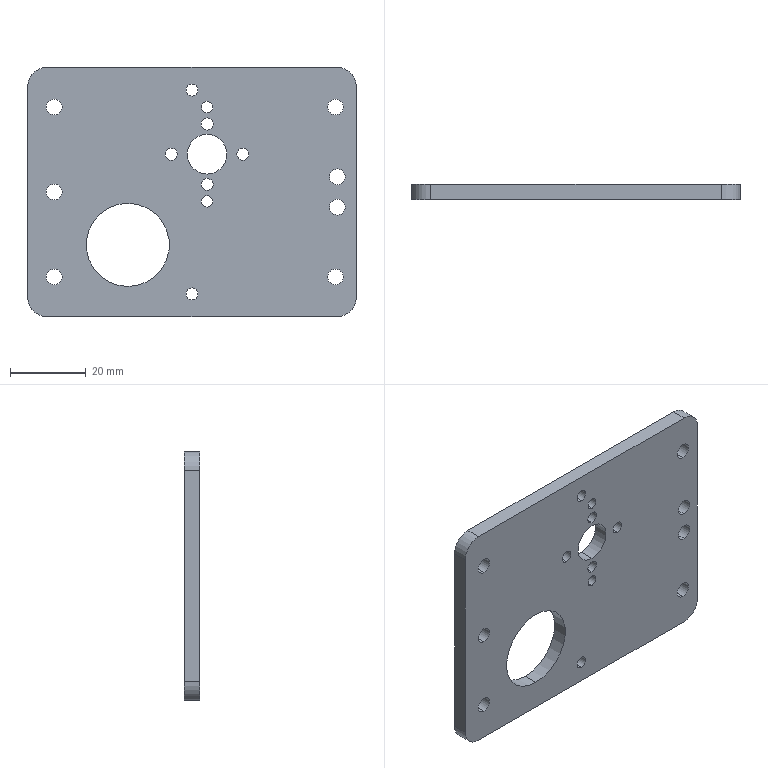Part | SolidWorks | features BaseBody 1 | 1 solid | 44 faces | box 87 x 4 x 66 mm | volume 20378 mm3 | cylinder 38 | plane 6 | commonest cylinder face diameters 4.2 x14 3.2 x12 3 x4 10 x4 10.5 x2 22 x2
STEP:
#1=CARTESIAN_POINT('',(38.5,4.,6.1));
#2=VERTEX_POINT('',#1);
#3=CARTESIAN_POINT('',(38.5,4.,1.9));
#4=VERTEX_POINT('',#3);
#5=CARTESIAN_POINT('',(38.5,4.,4.));
#6=DIRECTION('',(0.,-1.,0.));
#7=DIRECTION('',(0.,0.,-1.));
#8=AXIS2_PLACEMENT_3D('',#5,#6,#7);
#9=CIRCLE('',#8,2.1);
#10=EDGE_CURVE('',#2,#4,#9,.T.);
#11=ORIENTED_EDGE('',*,*,#10,.F.);
#12=CARTESIAN_POINT('',(38.5,0.,6.1));
#13=VERTEX_POINT('',#12);
#14=CARTESIAN_POINT('',(38.5,4.,6.1));
#15=DIRECTION('',(0.,-1.,0.));
#16=VECTOR('',#15,1000.);
#17=LINE('',#14,#16);
#18=EDGE_CURVE('',#2,#13,#17,.T.);
#19=ORIENTED_EDGE('',*,*,#18,.T.);
#20=CARTESIAN_POINT('',(38.5,0.,1.9));
#21=VERTEX_POINT('',#20);
#22=CARTESIAN_POINT('',(38.5,0.,4.));
#23=DIRECTION('',(0.,1.,0.));
#24=DIRECTION('',(0.,0.,-1.));
#25=AXIS2_PLACEMENT_3D('',#22,#23,#24);
#26=CIRCLE('',#25,2.1);
#27=EDGE_CURVE('',#21,#13,#26,.T.);
#28=ORIENTED_EDGE('',*,*,#27,.F.);
#29=CARTESIAN_POINT('',(38.5,4.,1.9));
#30=DIRECTION('',(0.,-1.,0.));
#31=VECTOR('',#30,1000.);
#32=LINE('',#29,#31);
#33=EDGE_CURVE('',#4,#21,#32,.T.);
#34=ORIENTED_EDGE('',*,*,#33,.F.);
#35=EDGE_LOOP('',(#11,#19,#28,#34));
#36=FACE_OUTER_BOUND('',#35,.T.);
#37=CARTESIAN_POINT('',(38.5,4.,4.));
#38=DIRECTION('',(0.,-1.,0.));
#39=DIRECTION('',(0.,0.,-1.));
#40=AXIS2_PLACEMENT_3D('',#37,#38,#39);
#41=CYLINDRICAL_SURFACE('',#40,2.1);
#42=ADVANCED_FACE('',(#36),#41,.F.);
#43=CARTESIAN_POINT('',(38.5,4.,-1.9));
#44=VERTEX_POINT('',#43);
#45=CARTESIAN_POINT('',(38.5,4.,-6.1));
#46=VERTEX_POINT('',#45);
#47=CARTESIAN_POINT('',(38.5,4.,-4.));
#48=DIRECTION('',(0.,-1.,0.));
#49=DIRECTION('',(0.,0.,-1.));
#50=AXIS2_PLACEMENT_3D('',#47,#48,#49);
#51=CIRCLE('',#50,2.1);
#52=EDGE_CURVE('',#44,#46,#51,.T.);
#53=ORIENTED_EDGE('',*,*,#52,.F.);
#54=CARTESIAN_POINT('',(38.5,0.,-1.9));
#55=VERTEX_POINT('',#54);
#56=CARTESIAN_POINT('',(38.5,4.,-1.9));
#57=DIRECTION('',(0.,-1.,0.));
#58=VECTOR('',#57,1000.);
#59=LINE('',#56,#58);
#60=EDGE_CURVE('',#44,#55,#59,.T.);
#61=ORIENTED_EDGE('',*,*,#60,.T.);
#62=CARTESIAN_POINT('',(38.5,0.,-6.1));
#63=VERTEX_POINT('',#62);
#64=CARTESIAN_POINT('',(38.5,0.,-4.));
#65=DIRECTION('',(0.,1.,0.));
#66=DIRECTION('',(0.,0.,-1.));
#67=AXIS2_PLACEMENT_3D('',#64,#65,#66);
#68=CIRCLE('',#67,2.1);
#69=EDGE_CURVE('',#63,#55,#68,.T.);
#70=ORIENTED_EDGE('',*,*,#69,.F.);
#71=CARTESIAN_POINT('',(38.5,4.,-6.1));
#72=DIRECTION('',(0.,-1.,0.));
#73=VECTOR('',#72,1000.);
#74=LINE('',#71,#73);
#75=EDGE_CURVE('',#46,#63,#74,.T.);
#76=ORIENTED_EDGE('',*,*,#75,.F.);
#77=EDGE_LOOP('',(#53,#61,#70,#76));
#78=FACE_OUTER_BOUND('',#77,.T.);
#79=CARTESIAN_POINT('',(38.5,4.,-4.));
#80=DIRECTION('',(0.,-1.,0.));
#81=DIRECTION('',(0.,0.,-1.));
#82=AXIS2_PLACEMENT_3D('',#79,#80,#81);
#83=CYLINDRICAL_SURFACE('',#82,2.1);
#84=ADVANCED_FACE('',(#78),#83,.F.);
#85=CARTESIAN_POINT('',(0.,4.,28.6));
#86=VERTEX_POINT('',#85);
#87=CARTESIAN_POINT('',(0.,4.,25.4));
#88=VERTEX_POINT('',#87);
#89=CARTESIAN_POINT('',(0.,4.,27.));
#90=DIRECTION('',(0.,-1.,0.));
#91=DIRECTION('',(0.,0.,-1.));
#92=AXIS2_PLACEMENT_3D('',#89,#90,#91);
#93=CIRCLE('',#92,1.6);
#94=EDGE_CURVE('',#86,#88,#93,.T.);
#95=ORIENTED_EDGE('',*,*,#94,.F.);
#96=CARTESIAN_POINT('',(0.,0.,28.6));
#97=VERTEX_POINT('',#96);
#98=CARTESIAN_POINT('',(0.,4.,28.6));
#99=DIRECTION('',(0.,-1.,0.));
#100=VECTOR('',#99,1000.);
#101=LINE('',#98,#100);
#102=EDGE_CURVE('',#86,#97,#101,.T.);
#103=ORIENTED_EDGE('',*,*,#102,.T.);
#104=CARTESIAN_POINT('',(0.,0.,25.4));
#105=VERTEX_POINT('',#104);
#106=CARTESIAN_POINT('',(0.,0.,27.));
#107=DIRECTION('',(0.,1.,0.));
#108=DIRECTION('',(0.,0.,-1.));
#109=AXIS2_PLACEMENT_3D('',#106,#107,#108);
#110=CIRCLE('',#109,1.6);
#111=EDGE_CURVE('',#105,#97,#110,.T.);
#112=ORIENTED_EDGE('',*,*,#111,.F.);
#113=CARTESIAN_POINT('',(0.,4.,25.4));
#114=DIRECTION('',(0.,-1.,0.));
#115=VECTOR('',#114,1000.);
#116=LINE('',#113,#115);
#117=EDGE_CURVE('',#88,#105,#116,.T.);
#118=ORIENTED_EDGE('',*,*,#117,.F.);
#119=EDGE_LOOP('',(#95,#103,#112,#118));
#120=FACE_OUTER_BOUND('',#119,.T.);
#121=CARTESIAN_POINT('',(0.,4.,27.));
#122=DIRECTION('',(0.,-1.,0.));
#123=DIRECTION('',(0.,0.,-1.));
#124=AXIS2_PLACEMENT_3D('',#121,#122,#123);
#125=CYLINDRICAL_SURFACE('',#124,1.6);
#126=ADVANCED_FACE('',(#120),#125,.F.);
#127=CARTESIAN_POINT('',(38.,4.,-20.4));
#128=VERTEX_POINT('',#127);
#129=CARTESIAN_POINT('',(38.,4.,-24.6));
#130=VERTEX_POINT('',#129);
#131=CARTESIAN_POINT('',(38.,4.,-22.5));
#132=DIRECTION('',(0.,-1.,0.));
#133=DIRECTION('',(0.,0.,-1.));
#134=AXIS2_PLACEMENT_3D('',#131,#132,#133);
#135=CIRCLE('',#134,2.1);
#136=EDGE_CURVE('',#128,#130,#135,.T.);
#137=ORIENTED_EDGE('',*,*,#136,.F.);
#138=CARTESIAN_POINT('',(38.,0.,-20.4));
#139=VERTEX_POINT('',#138);
#140=CARTESIAN_POINT('',(38.,4.,-20.4));
#141=DIRECTION('',(0.,-1.,0.));
#142=VECTOR('',#141,1000.);
#143=LINE('',#140,#142);
#144=EDGE_CURVE('',#128,#139,#143,.T.);
#145=ORIENTED_EDGE('',*,*,#144,.T.);
#146=CARTESIAN_POINT('',(38.,0.,-24.6));
#147=VERTEX_POINT('',#146);
#148=CARTESIAN_POINT('',(38.,0.,-22.5));
#149=DIRECTION('',(0.,1.,0.));
#150=DIRECTION('',(0.,0.,-1.));
#151=AXIS2_PLACEMENT_3D('',#148,#149,#150);
#152=CIRCLE('',#151,2.1);
#153=EDGE_CURVE('',#147,#139,#152,.T.);
#154=ORIENTED_EDGE('',*,*,#153,.F.);
#155=CARTESIAN_POINT('',(38.,4.,-24.6));
#156=DIRECTION('',(0.,-1.,0.));
#157=VECTOR('',#156,1000.);
#158=LINE('',#155,#157);
#159=EDGE_CURVE('',#130,#147,#158,.T.);
#160=ORIENTED_EDGE('',*,*,#159,.F.);
#161=EDGE_LOOP('',(#137,#145,#154,#160));
#162=FACE_OUTER_BOUND('',#161,.T.);
#163=CARTESIAN_POINT('',(38.,4.,-22.5));
#164=DIRECTION('',(0.,-1.,0.));
#165=DIRECTION('',(0.,0.,-1.));
#166=AXIS2_PLACEMENT_3D('',#163,#164,#165);
#167=CYLINDRICAL_SURFACE('',#166,2.1);
#168=ADVANCED_FACE('',(#162),#167,.F.);
#169=CARTESIAN_POINT('',(38.,4.,24.6));
#170=VERTEX_POINT('',#169);
#171=CARTESIAN_POINT('',(38.,4.,20.4));
#172=VERTEX_POINT('',#171);
#173=CARTESIAN_POINT('',(38.,4.,22.5));
#174=DIRECTION('',(0.,-1.,0.));
#175=DIRECTION('',(0.,0.,-1.));
#176=AXIS2_PLACEMENT_3D('',#173,#174,#175);
#177=CIRCLE('',#176,2.1);
#178=EDGE_CURVE('',#170,#172,#177,.T.);
#179=ORIENTED_EDGE('',*,*,#178,.F.);
#180=CARTESIAN_POINT('',(38.,0.,24.6));
#181=VERTEX_POINT('',#180);
#182=CARTESIAN_POINT('',(38.,4.,24.6));
#183=DIRECTION('',(0.,-1.,0.));
#184=VECTOR('',#183,1000.);
#185=LINE('',#182,#184);
#186=EDGE_CURVE('',#170,#181,#185,.T.);
#187=ORIENTED_EDGE('',*,*,#186,.T.);
#188=CARTESIAN_POINT('',(38.,0.,20.4));
#189=VERTEX_POINT('',#188);
#190=CARTESIAN_POINT('',(38.,0.,22.5));
#191=DIRECTION('',(0.,1.,0.));
#192=DIRECTION('',(0.,0.,-1.));
#193=AXIS2_PLACEMENT_3D('',#190,#191,#192);
#194=CIRCLE('',#193,2.1);
#195=EDGE_CURVE('',#189,#181,#194,.T.);
#196=ORIENTED_EDGE('',*,*,#195,.F.);
#197=CARTESIAN_POINT('',(38.,4.,20.4));
#198=DIRECTION('',(0.,-1.,0.));
#199=VECTOR('',#198,1000.);
#200=LINE('',#197,#199);
#201=EDGE_CURVE('',#172,#189,#200,.T.);
#202=ORIENTED_EDGE('',*,*,#201,.F.);
#203=EDGE_LOOP('',(#179,#187,#196,#202));
#204=FACE_OUTER_BOUND('',#203,.T.);
#205=CARTESIAN_POINT('',(38.,4.,22.5));
#206=DIRECTION('',(0.,-1.,0.));
#207=DIRECTION('',(0.,0.,-1.));
#208=AXIS2_PLACEMENT_3D('',#205,#206,#207);
#209=CYLINDRICAL_SURFACE('',#208,2.1);
#210=ADVANCED_FACE('',(#204),#209,.F.);
#211=CARTESIAN_POINT('',(-36.5,4.,24.6));
#212=VERTEX_POINT('',#211);
#213=CARTESIAN_POINT('',(-36.5,4.,20.4));
#214=VERTEX_POINT('',#213);
#215=CARTESIAN_POINT('',(-36.5,4.,22.5));
#216=DIRECTION('',(0.,-1.,0.));
#217=DIRECTION('',(0.,0.,-1.));
#218=AXIS2_PLACEMENT_3D('',#215,#216,#217);
#219=CIRCLE('',#218,2.1);
#220=EDGE_CURVE('',#212,#214,#219,.T.);
#221=ORIENTED_EDGE('',*,*,#220,.F.);
#222=CARTESIAN_POINT('',(-36.5,0.,24.6));
#223=VERTEX_POINT('',#222);
#224=CARTESIAN_POINT('',(-36.5,4.,24.6));
#225=DIRECTION('',(0.,-1.,0.));
#226=VECTOR('',#225,1000.);
#227=LINE('',#224,#226);
#228=EDGE_CURVE('',#212,#223,#227,.T.);
#229=ORIENTED_EDGE('',*,*,#228,.T.);
#230=CARTESIAN_POINT('',(-36.5,0.,20.4));
#231=VERTEX_POINT('',#230);
#232=CARTESIAN_POINT('',(-36.5,0.,22.5));
#233=DIRECTION('',(0.,1.,0.));
#234=DIRECTION('',(0.,0.,-1.));
#235=AXIS2_PLACEMENT_3D('',#232,#233,#234);
#236=CIRCLE('',#235,2.1);
#237=EDGE_CURVE('',#231,#223,#236,.T.);
#238=ORIENTED_EDGE('',*,*,#237,.F.);
#239=CARTESIAN_POINT('',(-36.5,4.,20.4));
#240=DIRECTION('',(0.,-1.,0.));
#241=VECTOR('',#240,1000.);
#242=LINE('',#239,#241);
#243=EDGE_CURVE('',#214,#231,#242,.T.);
#244=ORIENTED_EDGE('',*,*,#243,.F.);
#245=EDGE_LOOP('',(#221,#229,#238,#244));
#246=FACE_OUTER_BOUND('',#245,.T.);
#247=CARTESIAN_POINT('',(-36.5,4.,22.5));
#248=DIRECTION('',(0.,-1.,0.));
#249=DIRECTION('',(0.,0.,-1.));
#250=AXIS2_PLACEMENT_3D('',#247,#248,#249);
#251=CYLINDRICAL_SURFACE('',#250,2.1);
#252=ADVANCED_FACE('',(#246),#251,.F.);
#253=CARTESIAN_POINT('',(-36.5,4.,2.1));
#254=VERTEX_POINT('',#253);
#255=CARTESIAN_POINT('',(-36.5,4.,-2.1));
#256=VERTEX_POINT('',#255);
#257=CARTESIAN_POINT('',(-36.5,4.,0.));
#258=DIRECTION('',(0.,-1.,0.));
#259=DIRECTION('',(0.,0.,-1.));
#260=AXIS2_PLACEMENT_3D('',#257,#258,#259);
#261=CIRCLE('',#260,2.1);
#262=EDGE_CURVE('',#254,#256,#261,.T.);
#263=ORIENTED_EDGE('',*,*,#262,.F.);
#264=CARTESIAN_POINT('',(-36.5,0.,2.1));
#265=VERTEX_POINT('',#264);
#266=CARTESIAN_POINT('',(-36.5,4.,2.1));
#267=DIRECTION('',(0.,-1.,0.));
#268=VECTOR('',#267,1000.);
#269=LINE('',#266,#268);
#270=EDGE_CURVE('',#254,#265,#269,.T.);
#271=ORIENTED_EDGE('',*,*,#270,.T.);
#272=CARTESIAN_POINT('',(-36.5,0.,-2.1));
#273=VERTEX_POINT('',#272);
#274=CARTESIAN_POINT('',(-36.5,0.,0.));
#275=DIRECTION('',(0.,1.,0.));
#276=DIRECTION('',(0.,0.,-1.));
#277=AXIS2_PLACEMENT_3D('',#274,#275,#276);
#278=CIRCLE('',#277,2.1);
#279=EDGE_CURVE('',#273,#265,#278,.T.);
#280=ORIENTED_EDGE('',*,*,#279,.F.);
#281=CARTESIAN_POINT('',(-36.5,4.,-2.1));
#282=DIRECTION('',(0.,-1.,0.));
#283=VECTOR('',#282,1000.);
#284=LINE('',#281,#283);
#285=EDGE_CURVE('',#256,#273,#284,.T.);
#286=ORIENTED_EDGE('',*,*,#285,.F.);
#287=EDGE_LOOP('',(#263,#271,#280,#286));
#288=FACE_OUTER_BOUND('',#287,.T.);
#289=CARTESIAN_POINT('',(-36.5,4.,0.));
#290=DIRECTION('',(0.,-1.,0.));
#291=DIRECTION('',(0.,0.,-1.));
#292=AXIS2_PLACEMENT_3D('',#289,#290,#291);
#293=CYLINDRICAL_SURFACE('',#292,2.1);
#294=ADVANCED_FACE('',(#288),#293,.F.);
#295=CARTESIAN_POINT('',(-36.5,4.,-20.4));
#296=VERTEX_POINT('',#295);
#297=CARTESIAN_POINT('',(-36.5,4.,-24.6));
#298=VERTEX_POINT('',#297);
#299=CARTESIAN_POINT('',(-36.5,4.,-22.5));
#300=DIRECTION('',(0.,-1.,0.));
#301=DIRECTION('',(0.,0.,-1.));
#302=AXIS2_PLACEMENT_3D('',#299,#300,#301);
#303=CIRCLE('',#302,2.1);
#304=EDGE_CURVE('',#296,#298,#303,.T.);
#305=ORIENTED_EDGE('',*,*,#304,.F.);
#306=CARTESIAN_POINT('',(-36.5,0.,-20.4));
#307=VERTEX_POINT('',#306);
#308=CARTESIAN_POINT('',(-36.5,4.,-20.4));
#309=DIRECTION('',(0.,-1.,0.));
#310=VECTOR('',#309,1000.);
#311=LINE('',#308,#310);
#312=EDGE_CURVE('',#296,#307,#311,.T.);
#313=ORIENTED_EDGE('',*,*,#312,.T.);
#314=CARTESIAN_POINT('',(-36.5,0.,-24.6));
#315=VERTEX_POINT('',#314);
#316=CARTESIAN_POINT('',(-36.5,0.,-22.5));
#317=DIRECTION('',(0.,1.,0.));
#318=DIRECTION('',(0.,0.,-1.));
#319=AXIS2_PLACEMENT_3D('',#316,#317,#318);
#320=CIRCLE('',#319,2.1);
#321=EDGE_CURVE('',#315,#307,#320,.T.);
#322=ORIENTED_EDGE('',*,*,#321,.F.);
#323=CARTESIAN_POINT('',(-36.5,4.,-24.6));
#324=DIRECTION('',(0.,-1.,0.));
#325=VECTOR('',#324,1000.);
#326=LINE('',#323,#325);
#327=EDGE_CURVE('',#298,#315,#326,.T.);
#328=ORIENTED_EDGE('',*,*,#327,.F.);
#329=EDGE_LOOP('',(#305,#313,#322,#328));
#330=FACE_OUTER_BOUND('',#329,.T.);
#331=CARTESIAN_POINT('',(-36.5,4.,-22.5));
#332=DIRECTION('',(0.,-1.,0.));
#333=DIRECTION('',(0.,0.,-1.));
#334=AXIS2_PLACEMENT_3D('',#331,#332,#333);
#335=CYLINDRICAL_SURFACE('',#334,2.1);
#336=ADVANCED_FACE('',(#330),#335,.F.);
#337=CARTESIAN_POINT('',(0.,4.,-25.4));
#338=VERTEX_POINT('',#337);
#339=CARTESIAN_POINT('',(0.,4.,-28.6));
#340=VERTEX_POINT('',#339);
#341=CARTESIAN_POINT('',(0.,4.,-27.));
#342=DIRECTION('',(0.,-1.,0.));
#343=DIRECTION('',(0.,0.,-1.));
#344=AXIS2_PLACEMENT_3D('',#341,#342,#343);
#345=CIRCLE('',#344,1.6);
#346=EDGE_CURVE('',#338,#340,#345,.T.);
#347=ORIENTED_EDGE('',*,*,#346,.F.);
#348=CARTESIAN_POINT('',(0.,0.,-25.4));
#349=VERTEX_POINT('',#348);
#350=CARTESIAN_POINT('',(0.,4.,-25.4));
#351=DIRECTION('',(0.,-1.,0.));
#352=VECTOR('',#351,1000.);
#353=LINE('',#350,#352);
#354=EDGE_CURVE('',#338,#349,#353,.T.);
#355=ORIENTED_EDGE('',*,*,#354,.T.);
#356=CARTESIAN_POINT('',(0.,0.,-28.6));
#357=VERTEX_POINT('',#356);
#358=CARTESIAN_POINT('',(0.,0.,-27.));
#359=DIRECTION('',(0.,1.,0.));
#360=DIRECTION('',(0.,0.,-1.));
#361=AXIS2_PLACEMENT_3D('',#358,#359,#360);
#362=CIRCLE('',#361,1.6);
#363=EDGE_CURVE('',#357,#349,#362,.T.);
#364=ORIENTED_EDGE('',*,*,#363,.F.);
#365=CARTESIAN_POINT('',(0.,4.,-28.6));
#366=DIRECTION('',(0.,-1.,0.));
#367=VECTOR('',#366,1000.);
#368=LINE('',#365,#367);
#369=EDGE_CURVE('',#340,#357,#368,.T.);
#370=ORIENTED_EDGE('',*,*,#369,.F.);
#371=EDGE_LOOP('',(#347,#355,#364,#370));
#372=FACE_OUTER_BOUND('',#371,.T.);
#373=CARTESIAN_POINT('',(0.,4.,-27.));
#374=DIRECTION('',(0.,-1.,0.));
#375=DIRECTION('',(0.,0.,-1.));
#376=AXIS2_PLACEMENT_3D('',#373,#374,#375);
#377=CYLINDRICAL_SURFACE('',#376,1.6);
#378=ADVANCED_FACE('',(#372),#377,.F.);
#379=CARTESIAN_POINT('',(4.,4.,15.25));
#380=VERTEX_POINT('',#379);
#381=CARTESIAN_POINT('',(4.,4.,4.75));
#382=VERTEX_POINT('',#381);
#383=CARTESIAN_POINT('',(4.,4.,10.));
#384=DIRECTION('',(0.,-1.,0.));
#385=DIRECTION('',(0.,0.,-1.));
#386=AXIS2_PLACEMENT_3D('',#383,#384,#385);
#387=CIRCLE('',#386,5.25);
#388=EDGE_CURVE('',#380,#382,#387,.T.);
#389=ORIENTED_EDGE('',*,*,#388,.F.);
#390=CARTESIAN_POINT('',(4.,0.,15.25));
#391=VERTEX_POINT('',#390);
#392=CARTESIAN_POINT('',(4.,4.,15.25));
#393=DIRECTION('',(0.,-1.,0.));
#394=VECTOR('',#393,1000.);
#395=LINE('',#392,#394);
#396=EDGE_CURVE('',#380,#391,#395,.T.);
#397=ORIENTED_EDGE('',*,*,#396,.T.);
#398=CARTESIAN_POINT('',(4.,0.,4.75));
#399=VERTEX_POINT('',#398);
#400=CARTESIAN_POINT('',(4.,0.,10.));
#401=DIRECTION('',(0.,1.,0.));
#402=DIRECTION('',(0.,0.,-1.));
#403=AXIS2_PLACEMENT_3D('',#400,#401,#402);
#404=CIRCLE('',#403,5.25);
#405=EDGE_CURVE('',#399,#391,#404,.T.);
#406=ORIENTED_EDGE('',*,*,#405,.F.);
#407=CARTESIAN_POINT('',(4.,4.,4.75));
#408=DIRECTION('',(0.,-1.,0.));
#409=VECTOR('',#408,1000.);
#410=LINE('',#407,#409);
#411=EDGE_CURVE('',#382,#399,#410,.T.);
#412=ORIENTED_EDGE('',*,*,#411,.F.);
#413=EDGE_LOOP('',(#389,#397,#406,#412));
#414=FACE_OUTER_BOUND('',#413,.T.);
#415=CARTESIAN_POINT('',(4.,4.,10.));
#416=DIRECTION('',(0.,-1.,0.));
#417=DIRECTION('',(0.,0.,-1.));
#418=AXIS2_PLACEMENT_3D('',#415,#416,#417);
#419=CYLINDRICAL_SURFACE('',#418,5.25);
#420=ADVANCED_FACE('',(#414),#419,.F.);
#421=CARTESIAN_POINT('',(4.,4.,24.));
#422=VERTEX_POINT('',#421);
#423=CARTESIAN_POINT('',(4.,4.,21.));
#424=VERTEX_POINT('',#423);
#425=CARTESIAN_POINT('',(4.,4.,22.5));
#426=DIRECTION('',(0.,-1.,0.));
#427=DIRECTION('',(0.,0.,-1.));
#428=AXIS2_PLACEMENT_3D('',#425,#426,#427);
#429=CIRCLE('',#428,1.5);
#430=EDGE_CURVE('',#422,#424,#429,.T.);
#431=ORIENTED_EDGE('',*,*,#430,.F.);
#432=CARTESIAN_POINT('',(4.,0.,24.));
#433=VERTEX_POINT('',#432);
#434=CARTESIAN_POINT('',(4.,4.,24.));
#435=DIRECTION('',(0.,-1.,0.));
#436=VECTOR('',#435,1000.);
#437=LINE('',#434,#436);
#438=EDGE_CURVE('',#422,#433,#437,.T.);
#439=ORIENTED_EDGE('',*,*,#438,.T.);
#440=CARTESIAN_POINT('',(4.,0.,21.));
#441=VERTEX_POINT('',#440);
#442=CARTESIAN_POINT('',(4.,0.,22.5));
#443=DIRECTION('',(0.,1.,0.));
#444=DIRECTION('',(0.,0.,-1.));
#445=AXIS2_PLACEMENT_3D('',#442,#443,#444);
#446=CIRCLE('',#445,1.5);
#447=EDGE_CURVE('',#441,#433,#446,.T.);
#448=ORIENTED_EDGE('',*,*,#447,.F.);
#449=CARTESIAN_POINT('',(4.,4.,21.));
#450=DIRECTION('',(0.,-1.,0.));
#451=VECTOR('',#450,1000.);
#452=LINE('',#449,#451);
#453=EDGE_CURVE('',#424,#441,#452,.T.);
#454=ORIENTED_EDGE('',*,*,#453,.F.);
#455=EDGE_LOOP('',(#431,#439,#448,#454));
#456=FACE_OUTER_BOUND('',#455,.T.);
#457=CARTESIAN_POINT('',(4.,4.,22.5));
#458=DIRECTION('',(0.,-1.,0.));
#459=DIRECTION('',(0.,0.,-1.));
#460=AXIS2_PLACEMENT_3D('',#457,#458,#459);
#461=CYLINDRICAL_SURFACE('',#460,1.5);
#462=ADVANCED_FACE('',(#456),#461,.F.);
#463=CARTESIAN_POINT('',(4.,4.,-1.));
#464=VERTEX_POINT('',#463);
#465=CARTESIAN_POINT('',(4.,4.,-4.));
#466=VERTEX_POINT('',#465);
#467=CARTESIAN_POINT('',(4.,4.,-2.5));
#468=DIRECTION('',(0.,-1.,0.));
#469=DIRECTION('',(0.,0.,-1.));
#470=AXIS2_PLACEMENT_3D('',#467,#468,#469);
#471=CIRCLE('',#470,1.5);
#472=EDGE_CURVE('',#464,#466,#471,.T.);
#473=ORIENTED_EDGE('',*,*,#472,.F.);
#474=CARTESIAN_POINT('',(4.,0.,-1.));
#475=VERTEX_POINT('',#474);
#476=CARTESIAN_POINT('',(4.,4.,-1.));
#477=DIRECTION('',(0.,-1.,0.));
#478=VECTOR('',#477,1000.);
#479=LINE('',#476,#478);
#480=EDGE_CURVE('',#464,#475,#479,.T.);
#481=ORIENTED_EDGE('',*,*,#480,.T.);
#482=CARTESIAN_POINT('',(4.,0.,-4.));
#483=VERTEX_POINT('',#482);
#484=CARTESIAN_POINT('',(4.,0.,-2.5));
#485=DIRECTION('',(0.,1.,0.));
#486=DIRECTION('',(0.,0.,-1.));
#487=AXIS2_PLACEMENT_3D('',#484,#485,#486);
#488=CIRCLE('',#487,1.5);
#489=EDGE_CURVE('',#483,#475,#488,.T.);
#490=ORIENTED_EDGE('',*,*,#489,.F.);
#491=CARTESIAN_POINT('',(4.,4.,-4.));
#492=DIRECTION('',(0.,-1.,0.));
#493=VECTOR('',#492,1000.);
#494=LINE('',#491,#493);
#495=EDGE_CURVE('',#466,#483,#494,.T.);
#496=ORIENTED_EDGE('',*,*,#495,.F.);
#497=EDGE_LOOP('',(#473,#481,#490,#496));
#498=FACE_OUTER_BOUND('',#497,.T.);
#499=CARTESIAN_POINT('',(4.,4.,-2.5));
#500=DIRECTION('',(0.,-1.,0.));
#501=DIRECTION('',(0.,0.,-1.));
#502=AXIS2_PLACEMENT_3D('',#499,#500,#501);
#503=CYLINDRICAL_SURFACE('',#502,1.5);
#504=ADVANCED_FACE('',(#498),#503,.F.);
#505=CARTESIAN_POINT('',(4.,4.,3.6));
#506=VERTEX_POINT('',#505);
#507=CARTESIAN_POINT('',(4.,4.,0.4));
#508=VERTEX_POINT('',#507);
#509=CARTESIAN_POINT('',(4.,4.,2.));
#510=DIRECTION('',(0.,-1.,0.));
#511=DIRECTION('',(0.,0.,-1.));
#512=AXIS2_PLACEMENT_3D('',#509,#510,#511);
#513=CIRCLE('',#512,1.6);
#514=EDGE_CURVE('',#506,#508,#513,.T.);
#515=ORIENTED_EDGE('',*,*,#514,.F.);
#516=CARTESIAN_POINT('',(4.,0.,3.6));
#517=VERTEX_POINT('',#516);
#518=CARTESIAN_POINT('',(4.,4.,3.6));
#519=DIRECTION('',(0.,-1.,0.));
#520=VECTOR('',#519,1000.);
#521=LINE('',#518,#520);
#522=EDGE_CURVE('',#506,#517,#521,.T.);
#523=ORIENTED_EDGE('',*,*,#522,.T.);
#524=CARTESIAN_POINT('',(4.,0.,0.4));
#525=VERTEX_POINT('',#524);
#526=CARTESIAN_POINT('',(4.,0.,2.));
#527=DIRECTION('',(0.,1.,0.));
#528=DIRECTION('',(0.,0.,-1.));
#529=AXIS2_PLACEMENT_3D('',#526,#527,#528);
#530=CIRCLE('',#529,1.6);
#531=EDGE_CURVE('',#525,#517,#530,.T.);
#532=ORIENTED_EDGE('',*,*,#531,.F.);
#533=CARTESIAN_POINT('',(4.,4.,0.4));
#534=DIRECTION('',(0.,-1.,0.));
#535=VECTOR('',#534,1000.);
#536=LINE('',#533,#535);
#537=EDGE_CURVE('',#508,#525,#536,.T.);
#538=ORIENTED_EDGE('',*,*,#537,.F.);
#539=EDGE_LOOP('',(#515,#523,#532,#538));
#540=FACE_OUTER_BOUND('',#539,.T.);
#541=CARTESIAN_POINT('',(4.,4.,2.));
#542=DIRECTION('',(0.,-1.,0.));
#543=DIRECTION('',(0.,0.,-1.));
#544=AXIS2_PLACEMENT_3D('',#541,#542,#543);
#545=CYLINDRICAL_SURFACE('',#544,1.6);
#546=ADVANCED_FACE('',(#540),#545,.F.);
#547=CARTESIAN_POINT('',(4.,4.,19.6));
#548=VERTEX_POINT('',#547);
#549=CARTESIAN_POINT('',(4.,4.,16.4));
#550=VERTEX_POINT('',#549);
#551=CARTESIAN_POINT('',(4.,4.,18.));
#552=DIRECTION('',(0.,-1.,0.));
#553=DIRECTION('',(0.,0.,-1.));
#554=AXIS2_PLACEMENT_3D('',#551,#552,#553);
#555=CIRCLE('',#554,1.6);
#556=EDGE_CURVE('',#548,#550,#555,.T.);
#557=ORIENTED_EDGE('',*,*,#556,.F.);
#558=CARTESIAN_POINT('',(4.,0.,19.6));
#559=VERTEX_POINT('',#558);
#560=CARTESIAN_POINT('',(4.,4.,19.6));
#561=DIRECTION('',(0.,-1.,0.));
#562=VECTOR('',#561,1000.);
#563=LINE('',#560,#562);
#564=EDGE_CURVE('',#548,#559,#563,.T.);
#565=ORIENTED_EDGE('',*,*,#564,.T.);
#566=CARTESIAN_POINT('',(4.,0.,16.4));
#567=VERTEX_POINT('',#566);
#568=CARTESIAN_POINT('',(4.,0.,18.));
#569=DIRECTION('',(0.,1.,0.));
#570=DIRECTION('',(0.,0.,-1.));
#571=AXIS2_PLACEMENT_3D('',#568,#569,#570);
#572=CIRCLE('',#571,1.6);
#573=EDGE_CURVE('',#567,#559,#572,.T.);
#574=ORIENTED_EDGE('',*,*,#573,.F.);
#575=CARTESIAN_POINT('',(4.,4.,16.4));
#576=DIRECTION('',(0.,-1.,0.));
#577=VECTOR('',#576,1000.);
#578=LINE('',#575,#577);
#579=EDGE_CURVE('',#550,#567,#578,.T.);
#580=ORIENTED_EDGE('',*,*,#579,.F.);
#581=EDGE_LOOP('',(#557,#565,#574,#580));
#582=FACE_OUTER_BOUND('',#581,.T.);
#583=CARTESIAN_POINT('',(4.,4.,18.));
#584=DIRECTION('',(0.,-1.,0.));
#585=DIRECTION('',(0.,0.,-1.));
#586=AXIS2_PLACEMENT_3D('',#583,#584,#585);
#587=CYLINDRICAL_SURFACE('',#586,1.6);
#588=ADVANCED_FACE('',(#582),#587,.F.);
#589=CARTESIAN_POINT('',(13.5,4.,11.6));
#590=VERTEX_POINT('',#589);
#591=CARTESIAN_POINT('',(13.5,4.,8.4));
#592=VERTEX_POINT('',#591);
#593=CARTESIAN_POINT('',(13.5,4.,10.));
#594=DIRECTION('',(0.,-1.,0.));
#595=DIRECTION('',(0.,0.,-1.));
#596=AXIS2_PLACEMENT_3D('',#593,#594,#595);
#597=CIRCLE('',#596,1.6);
#598=EDGE_CURVE('',#590,#592,#597,.T.);
#599=ORIENTED_EDGE('',*,*,#598,.F.);
#600=CARTESIAN_POINT('',(13.5,0.,11.6));
#601=VERTEX_POINT('',#600);
#602=CARTESIAN_POINT('',(13.5,4.,11.6));
#603=DIRECTION('',(0.,-1.,0.));
#604=VECTOR('',#603,1000.);
#605=LINE('',#602,#604);
#606=EDGE_CURVE('',#590,#601,#605,.T.);
#607=ORIENTED_EDGE('',*,*,#606,.T.);
#608=CARTESIAN_POINT('',(13.5,0.,8.4));
#609=VERTEX_POINT('',#608);
#610=CARTESIAN_POINT('',(13.5,0.,10.));
#611=DIRECTION('',(0.,1.,0.));
#612=DIRECTION('',(0.,0.,-1.));
#613=AXIS2_PLACEMENT_3D('',#610,#611,#612);
#614=CIRCLE('',#613,1.6);
#615=EDGE_CURVE('',#609,#601,#614,.T.);
#616=ORIENTED_EDGE('',*,*,#615,.F.);
#617=CARTESIAN_POINT('',(13.5,4.,8.4));
#618=DIRECTION('',(0.,-1.,0.));
#619=VECTOR('',#618,1000.);
#620=LINE('',#617,#619);
#621=EDGE_CURVE('',#592,#609,#620,.T.);
#622=ORIENTED_EDGE('',*,*,#621,.F.);
#623=EDGE_LOOP('',(#599,#607,#616,#622));
#624=FACE_OUTER_BOUND('',#623,.T.);
#625=CARTESIAN_POINT('',(13.5,4.,10.));
#626=DIRECTION('',(0.,-1.,0.));
#627=DIRECTION('',(0.,0.,-1.));
#628=AXIS2_PLACEMENT_3D('',#625,#626,#627);
#629=CYLINDRICAL_SURFACE('',#628,1.6);
#630=ADVANCED_FACE('',(#624),#629,.F.);
#631=CARTESIAN_POINT('',(-5.5,4.,11.6));
#632=VERTEX_POINT('',#631);
#633=CARTESIAN_POINT('',(-5.5,4.,8.4));
#634=VERTEX_POINT('',#633);
#635=CARTESIAN_POINT('',(-5.5,4.,10.));
#636=DIRECTION('',(0.,-1.,0.));
#637=DIRECTION('',(0.,0.,-1.));
#638=AXIS2_PLACEMENT_3D('',#635,#636,#637);
#639=CIRCLE('',#638,1.6);
#640=EDGE_CURVE('',#632,#634,#639,.T.);
#641=ORIENTED_EDGE('',*,*,#640,.F.);
#642=CARTESIAN_POINT('',(-5.5,0.,11.6));
#643=VERTEX_POINT('',#642);
#644=CARTESIAN_POINT('',(-5.5,4.,11.6));
#645=DIRECTION('',(0.,-1.,0.));
#646=VECTOR('',#645,1000.);
#647=LINE('',#644,#646);
#648=EDGE_CURVE('',#632,#643,#647,.T.);
#649=ORIENTED_EDGE('',*,*,#648,.T.);
#650=CARTESIAN_POINT('',(-5.5,0.,8.4));
#651=VERTEX_POINT('',#650);
#652=CARTESIAN_POINT('',(-5.5,0.,10.));
#653=DIRECTION('',(0.,1.,0.));
#654=DIRECTION('',(0.,0.,-1.));
#655=AXIS2_PLACEMENT_3D('',#652,#653,#654);
#656=CIRCLE('',#655,1.6);
#657=EDGE_CURVE('',#651,#643,#656,.T.);
#658=ORIENTED_EDGE('',*,*,#657,.F.);
#659=CARTESIAN_POINT('',(-5.5,4.,8.4));
#660=DIRECTION('',(0.,-1.,0.));
#661=VECTOR('',#660,1000.);
#662=LINE('',#659,#661);
#663=EDGE_CURVE('',#634,#651,#662,.T.);
#664=ORIENTED_EDGE('',*,*,#663,.F.);
#665=EDGE_LOOP('',(#641,#649,#658,#664));
#666=FACE_OUTER_BOUND('',#665,.T.);
#667=CARTESIAN_POINT('',(-5.5,4.,10.));
#668=DIRECTION('',(0.,-1.,0.));
#669=DIRECTION('',(0.,0.,-1.));
#670=AXIS2_PLACEMENT_3D('',#667,#668,#669);
#671=CYLINDRICAL_SURFACE('',#670,1.6);
#672=ADVANCED_FACE('',(#666),#671,.F.);
#673=CARTESIAN_POINT('',(-17.,0.,-25.));
#674=VERTEX_POINT('',#673);
#675=CARTESIAN_POINT('',(-17.,0.,-3.));
#676=VERTEX_POINT('',#675);
#677=CARTESIAN_POINT('',(-17.,0.,-14.));
#678=DIRECTION('',(0.,1.,0.));
#679=DIRECTION('',(0.,0.,1.));
#680=AXIS2_PLACEMENT_3D('',#677,#678,#679);
#681=CIRCLE('',#680,11.);
#682=EDGE_CURVE('',#674,#676,#681,.T.);
#683=ORIENTED_EDGE('',*,*,#682,.F.);
#684=CARTESIAN_POINT('',(-17.,4.,-25.));
#685=VERTEX_POINT('',#684);
#686=CARTESIAN_POINT('',(-17.,-6.,-25.));
#687=DIRECTION('',(0.,1.,0.));
#688=VECTOR('',#687,1000.);
#689=LINE('',#686,#688);
#690=EDGE_CURVE('',#674,#685,#689,.T.);
#691=ORIENTED_EDGE('',*,*,#690,.T.);
#692=CARTESIAN_POINT('',(-17.,4.,-3.));
#693=VERTEX_POINT('',#692);
#694=CARTESIAN_POINT('',(-17.,4.,-14.));
#695=DIRECTION('',(0.,-1.,0.));
#696=DIRECTION('',(0.,0.,1.));
#697=AXIS2_PLACEMENT_3D('',#694,#695,#696);
#698=CIRCLE('',#697,11.);
#699=EDGE_CURVE('',#693,#685,#698,.T.);
#700=ORIENTED_EDGE('',*,*,#699,.F.);
#701=CARTESIAN_POINT('',(-17.,-6.,-3.));
#702=DIRECTION('',(0.,1.,0.));
#703=VECTOR('',#702,1000.);
#704=LINE('',#701,#703);
#705=EDGE_CURVE('',#676,#693,#704,.T.);
#706=ORIENTED_EDGE('',*,*,#705,.F.);
#707=EDGE_LOOP('',(#683,#691,#700,#706));
#708=FACE_OUTER_BOUND('',#707,.T.);
#709=CARTESIAN_POINT('',(-17.,-6.,-14.));
#710=DIRECTION('',(0.,1.,0.));
#711=DIRECTION('',(0.,0.,1.));
#712=AXIS2_PLACEMENT_3D('',#709,#710,#711);
#713=CYLINDRICAL_SURFACE('',#712,11.);
#714=ADVANCED_FACE('',(#708),#713,.F.);
#715=CARTESIAN_POINT('',(38.5,4.,4.));
#716=DIRECTION('',(0.,-1.,0.));
#717=DIRECTION('',(0.,0.,-1.));
#718=AXIS2_PLACEMENT_3D('',#715,#716,#717);
#719=CIRCLE('',#718,2.1);
#720=EDGE_CURVE('',#4,#2,#719,.T.);
#721=ORIENTED_EDGE('',*,*,#720,.T.);
#722=ORIENTED_EDGE('',*,*,#10,.T.);
#723=EDGE_LOOP('',(#721,#722));
#724=FACE_BOUND('',#723,.T.);
#725=CARTESIAN_POINT('',(38.5,4.,-4.));
#726=DIRECTION('',(0.,-1.,0.));
#727=DIRECTION('',(0.,0.,-1.));
#728=AXIS2_PLACEMENT_3D('',#725,#726,#727);
#729=CIRCLE('',#728,2.1);
#730=EDGE_CURVE('',#46,#44,#729,.T.);
#731=ORIENTED_EDGE('',*,*,#730,.T.);
#732=ORIENTED_EDGE('',*,*,#52,.T.);
#733=EDGE_LOOP('',(#731,#732));
#734=FACE_BOUND('',#733,.T.);
#735=CARTESIAN_POINT('',(0.,4.,27.));
#736=DIRECTION('',(0.,-1.,0.));
#737=DIRECTION('',(0.,0.,-1.));
#738=AXIS2_PLACEMENT_3D('',#735,#736,#737);
#739=CIRCLE('',#738,1.6);
#740=EDGE_CURVE('',#88,#86,#739,.T.);
#741=ORIENTED_EDGE('',*,*,#740,.T.);
#742=ORIENTED_EDGE('',*,*,#94,.T.);
#743=EDGE_LOOP('',(#741,#742));
#744=FACE_BOUND('',#743,.T.);
#745=CARTESIAN_POINT('',(38.,4.,-22.5));
#746=DIRECTION('',(0.,-1.,0.));
#747=DIRECTION('',(0.,0.,-1.));
#748=AXIS2_PLACEMENT_3D('',#745,#746,#747);
#749=CIRCLE('',#748,2.1);
#750=EDGE_CURVE('',#130,#128,#749,.T.);
#751=ORIENTED_EDGE('',*,*,#750,.T.);
#752=ORIENTED_EDGE('',*,*,#136,.T.);
#753=EDGE_LOOP('',(#751,#752));
#754=FACE_BOUND('',#753,.T.);
#755=CARTESIAN_POINT('',(38.,4.,22.5));
#756=DIRECTION('',(0.,-1.,0.));
#757=DIRECTION('',(0.,0.,-1.));
#758=AXIS2_PLACEMENT_3D('',#755,#756,#757);
#759=CIRCLE('',#758,2.1);
#760=EDGE_CURVE('',#172,#170,#759,.T.);
#761=ORIENTED_EDGE('',*,*,#760,.T.);
#762=ORIENTED_EDGE('',*,*,#178,.T.);
#763=EDGE_LOOP('',(#761,#762));
#764=FACE_BOUND('',#763,.T.);
#765=CARTESIAN_POINT('',(-36.5,4.,22.5));
#766=DIRECTION('',(0.,-1.,0.));
#767=DIRECTION('',(0.,0.,-1.));
#768=AXIS2_PLACEMENT_3D('',#765,#766,#767);
#769=CIRCLE('',#768,2.1);
#770=EDGE_CURVE('',#214,#212,#769,.T.);
#771=ORIENTED_EDGE('',*,*,#770,.T.);
#772=ORIENTED_EDGE('',*,*,#220,.T.);
#773=EDGE_LOOP('',(#771,#772));
#774=FACE_BOUND('',#773,.T.);
#775=CARTESIAN_POINT('',(-36.5,4.,0.));
#776=DIRECTION('',(0.,-1.,0.));
#777=DIRECTION('',(0.,0.,-1.));
#778=AXIS2_PLACEMENT_3D('',#775,#776,#777);
#779=CIRCLE('',#778,2.1);
#780=EDGE_CURVE('',#256,#254,#779,.T.);
#781=ORIENTED_EDGE('',*,*,#780,.T.);
#782=ORIENTED_EDGE('',*,*,#262,.T.);
#783=EDGE_LOOP('',(#781,#782));
#784=FACE_BOUND('',#783,.T.);
#785=CARTESIAN_POINT('',(-36.5,4.,-22.5));
#786=DIRECTION('',(0.,-1.,0.));
#787=DIRECTION('',(0.,0.,-1.));
#788=AXIS2_PLACEMENT_3D('',#785,#786,#787);
#789=CIRCLE('',#788,2.1);
#790=EDGE_CURVE('',#298,#296,#789,.T.);
#791=ORIENTED_EDGE('',*,*,#790,.T.);
#792=ORIENTED_EDGE('',*,*,#304,.T.);
#793=EDGE_LOOP('',(#791,#792));
#794=FACE_BOUND('',#793,.T.);
#795=CARTESIAN_POINT('',(0.,4.,-27.));
#796=DIRECTION('',(0.,-1.,0.));
#797=DIRECTION('',(0.,0.,-1.));
#798=AXIS2_PLACEMENT_3D('',#795,#796,#797);
#799=CIRCLE('',#798,1.6);
#800=EDGE_CURVE('',#340,#338,#799,.T.);
#801=ORIENTED_EDGE('',*,*,#800,.T.);
#802=ORIENTED_EDGE('',*,*,#346,.T.);
#803=EDGE_LOOP('',(#801,#802));
#804=FACE_BOUND('',#803,.T.);
#805=CARTESIAN_POINT('',(-38.5,4.,33.));
#806=VERTEX_POINT('',#805);
#807=CARTESIAN_POINT('',(38.5,4.,33.));
#808=VERTEX_POINT('',#807);
#809=CARTESIAN_POINT('',(0.,4.,33.));
#810=DIRECTION('',(1.,0.,0.));
#811=VECTOR('',#810,1000.);
#812=LINE('',#809,#811);
#813=EDGE_CURVE('',#806,#808,#812,.T.);
#814=ORIENTED_EDGE('',*,*,#813,.T.);
#815=CARTESIAN_POINT('',(43.5,4.,28.));
#816=VERTEX_POINT('',#815);
#817=CARTESIAN_POINT('',(38.5,4.,28.));
#818=DIRECTION('',(0.,1.,0.));
#819=DIRECTION('',(0.,0.,-1.));
#820=AXIS2_PLACEMENT_3D('',#817,#818,#819);
#821=CIRCLE('',#820,5.);
#822=EDGE_CURVE('',#808,#816,#821,.T.);
#823=ORIENTED_EDGE('',*,*,#822,.T.);
#824=CARTESIAN_POINT('',(43.5,4.,-28.));
#825=VERTEX_POINT('',#824);
#826=CARTESIAN_POINT('',(43.5,4.,0.));
#827=DIRECTION('',(0.,0.,-1.));
#828=VECTOR('',#827,1000.);
#829=LINE('',#826,#828);
#830=EDGE_CURVE('',#816,#825,#829,.T.);
#831=ORIENTED_EDGE('',*,*,#830,.T.);
#832=CARTESIAN_POINT('',(38.5,4.,-33.));
#833=VERTEX_POINT('',#832);
#834=CARTESIAN_POINT('',(38.5,4.,-28.));
#835=DIRECTION('',(0.,1.,0.));
#836=DIRECTION('',(0.,0.,-1.));
#837=AXIS2_PLACEMENT_3D('',#834,#835,#836);
#838=CIRCLE('',#837,5.);
#839=EDGE_CURVE('',#825,#833,#838,.T.);
#840=ORIENTED_EDGE('',*,*,#839,.T.);
#841=CARTESIAN_POINT('',(-38.5,4.,-33.));
#842=VERTEX_POINT('',#841);
#843=CARTESIAN_POINT('',(0.,4.,-33.));
#844=DIRECTION('',(-1.,0.,0.));
#845=VECTOR('',#844,1000.);
#846=LINE('',#843,#845);
#847=EDGE_CURVE('',#833,#842,#846,.T.);
#848=ORIENTED_EDGE('',*,*,#847,.T.);
#849=CARTESIAN_POINT('',(-43.5,4.,-28.));
#850=VERTEX_POINT('',#849);
#851=CARTESIAN_POINT('',(-38.5,4.,-28.));
#852=DIRECTION('',(0.,1.,0.));
#853=DIRECTION('',(0.,0.,-1.));
#854=AXIS2_PLACEMENT_3D('',#851,#852,#853);
#855=CIRCLE('',#854,5.);
#856=EDGE_CURVE('',#842,#850,#855,.T.);
#857=ORIENTED_EDGE('',*,*,#856,.T.);
#858=CARTESIAN_POINT('',(-43.5,4.,28.));
#859=VERTEX_POINT('',#858);
#860=CARTESIAN_POINT('',(-43.5,4.,0.));
#861=DIRECTION('',(0.,0.,1.));
#862=VECTOR('',#861,1000.);
#863=LINE('',#860,#862);
#864=EDGE_CURVE('',#850,#859,#863,.T.);
#865=ORIENTED_EDGE('',*,*,#864,.T.);
#866=CARTESIAN_POINT('',(-38.5,4.,28.));
#867=DIRECTION('',(0.,1.,0.));
#868=DIRECTION('',(0.,0.,-1.));
#869=AXIS2_PLACEMENT_3D('',#866,#867,#868);
#870=CIRCLE('',#869,5.);
#871=EDGE_CURVE('',#859,#806,#870,.T.);
#872=ORIENTED_EDGE('',*,*,#871,.T.);
#873=EDGE_LOOP('',(#814,#823,#831,#840,#848,#857,#865,#872));
#874=FACE_OUTER_BOUND('',#873,.T.);
#875=CARTESIAN_POINT('',(4.,4.,10.));
#876=DIRECTION('',(0.,-1.,0.));
#877=DIRECTION('',(0.,0.,-1.));
#878=AXIS2_PLACEMENT_3D('',#875,#876,#877);
#879=CIRCLE('',#878,5.25);
#880=EDGE_CURVE('',#382,#380,#879,.T.);
#881=ORIENTED_EDGE('',*,*,#880,.T.);
#882=ORIENTED_EDGE('',*,*,#388,.T.);
#883=EDGE_LOOP('',(#881,#882));
#884=FACE_BOUND('',#883,.T.);
#885=CARTESIAN_POINT('',(4.,4.,22.5));
#886=DIRECTION('',(0.,-1.,0.));
#887=DIRECTION('',(0.,0.,-1.));
#888=AXIS2_PLACEMENT_3D('',#885,#886,#887);
#889=CIRCLE('',#888,1.5);
#890=EDGE_CURVE('',#424,#422,#889,.T.);
#891=ORIENTED_EDGE('',*,*,#890,.T.);
#892=ORIENTED_EDGE('',*,*,#430,.T.);
#893=EDGE_LOOP('',(#891,#892));
#894=FACE_BOUND('',#893,.T.);
#895=CARTESIAN_POINT('',(4.,4.,-2.5));
#896=DIRECTION('',(0.,-1.,0.));
#897=DIRECTION('',(0.,0.,-1.));
#898=AXIS2_PLACEMENT_3D('',#895,#896,#897);
#899=CIRCLE('',#898,1.5);
#900=EDGE_CURVE('',#466,#464,#899,.T.);
#901=ORIENTED_EDGE('',*,*,#900,.T.);
#902=ORIENTED_EDGE('',*,*,#472,.T.);
#903=EDGE_LOOP('',(#901,#902));
#904=FACE_BOUND('',#903,.T.);
#905=CARTESIAN_POINT('',(4.,4.,2.));
#906=DIRECTION('',(0.,-1.,0.));
#907=DIRECTION('',(0.,0.,-1.));
#908=AXIS2_PLACEMENT_3D('',#905,#906,#907);
#909=CIRCLE('',#908,1.6);
#910=EDGE_CURVE('',#508,#506,#909,.T.);
#911=ORIENTED_EDGE('',*,*,#910,.T.);
#912=ORIENTED_EDGE('',*,*,#514,.T.);
#913=EDGE_LOOP('',(#911,#912));
#914=FACE_BOUND('',#913,.T.);
#915=CARTESIAN_POINT('',(4.,4.,18.));
#916=DIRECTION('',(0.,-1.,0.));
#917=DIRECTION('',(0.,0.,-1.));
#918=AXIS2_PLACEMENT_3D('',#915,#916,#917);
#919=CIRCLE('',#918,1.6);
#920=EDGE_CURVE('',#550,#548,#919,.T.);
#921=ORIENTED_EDGE('',*,*,#920,.T.);
#922=ORIENTED_EDGE('',*,*,#556,.T.);
#923=EDGE_LOOP('',(#921,#922));
#924=FACE_BOUND('',#923,.T.);
#925=CARTESIAN_POINT('',(13.5,4.,10.));
#926=DIRECTION('',(0.,-1.,0.));
#927=DIRECTION('',(0.,0.,-1.));
#928=AXIS2_PLACEMENT_3D('',#925,#926,#927);
#929=CIRCLE('',#928,1.6);
#930=EDGE_CURVE('',#592,#590,#929,.T.);
#931=ORIENTED_EDGE('',*,*,#930,.T.);
#932=ORIENTED_EDGE('',*,*,#598,.T.);
#933=EDGE_LOOP('',(#931,#932));
#934=FACE_BOUND('',#933,.T.);
#935=CARTESIAN_POINT('',(-5.5,4.,10.));
#936=DIRECTION('',(0.,-1.,0.));
#937=DIRECTION('',(0.,0.,-1.));
#938=AXIS2_PLACEMENT_3D('',#935,#936,#937);
#939=CIRCLE('',#938,1.6);
#940=EDGE_CURVE('',#634,#632,#939,.T.);
#941=ORIENTED_EDGE('',*,*,#940,.T.);
#942=ORIENTED_EDGE('',*,*,#640,.T.);
#943=EDGE_LOOP('',(#941,#942));
#944=FACE_BOUND('',#943,.T.);
#945=ORIENTED_EDGE('',*,*,#699,.T.);
#946=CARTESIAN_POINT('',(-17.,4.,-14.));
#947=DIRECTION('',(0.,-1.,0.));
#948=DIRECTION('',(0.,0.,1.));
#949=AXIS2_PLACEMENT_3D('',#946,#947,#948);
#950=CIRCLE('',#949,11.);
#951=EDGE_CURVE('',#685,#693,#950,.T.);
#952=ORIENTED_EDGE('',*,*,#951,.T.);
#953=EDGE_LOOP('',(#945,#952));
#954=FACE_BOUND('',#953,.T.);
#955=CARTESIAN_POINT('',(0.,4.,0.));
#956=DIRECTION('',(0.,1.,0.));
#957=DIRECTION('',(0.,0.,1.));
#958=AXIS2_PLACEMENT_3D('',#955,#956,#957);
#959=PLANE('',#958);
#960=ADVANCED_FACE('',(#724,#734,#744,#754,#764,#774,#784,#794,#804,#874,#884,#894,#904,#914,#924,#934,#944,#954),#959,.T.);
#961=ORIENTED_EDGE('',*,*,#18,.F.);
#962=ORIENTED_EDGE('',*,*,#720,.F.);
#963=ORIENTED_EDGE('',*,*,#33,.T.);
#964=CARTESIAN_POINT('',(38.5,0.,4.));
#965=DIRECTION('',(0.,1.,0.));
#966=DIRECTION('',(0.,0.,-1.));
#967=AXIS2_PLACEMENT_3D('',#964,#965,#966);
#968=CIRCLE('',#967,2.1);
#969=EDGE_CURVE('',#13,#21,#968,.T.);
#970=ORIENTED_EDGE('',*,*,#969,.F.);
#971=EDGE_LOOP('',(#961,#962,#963,#970));
#972=FACE_OUTER_BOUND('',#971,.T.);
#973=CARTESIAN_POINT('',(38.5,4.,4.));
#974=DIRECTION('',(0.,-1.,0.));
#975=DIRECTION('',(0.,0.,-1.));
#976=AXIS2_PLACEMENT_3D('',#973,#974,#975);
#977=CYLINDRICAL_SURFACE('',#976,2.1);
#978=ADVANCED_FACE('',(#972),#977,.F.);
#979=ORIENTED_EDGE('',*,*,#60,.F.);
#980=ORIENTED_EDGE('',*,*,#730,.F.);
#981=ORIENTED_EDGE('',*,*,#75,.T.);
#982=CARTESIAN_POINT('',(38.5,0.,-4.));
#983=DIRECTION('',(0.,1.,0.));
#984=DIRECTION('',(0.,0.,-1.));
#985=AXIS2_PLACEMENT_3D('',#982,#983,#984);
#986=CIRCLE('',#985,2.1);
#987=EDGE_CURVE('',#55,#63,#986,.T.);
#988=ORIENTED_EDGE('',*,*,#987,.F.);
#989=EDGE_LOOP('',(#979,#980,#981,#988));
#990=FACE_OUTER_BOUND('',#989,.T.);
#991=CARTESIAN_POINT('',(38.5,4.,-4.));
#992=DIRECTION('',(0.,-1.,0.));
#993=DIRECTION('',(0.,0.,-1.));
#994=AXIS2_PLACEMENT_3D('',#991,#992,#993);
#995=CYLINDRICAL_SURFACE('',#994,2.1);
#996=ADVANCED_FACE('',(#990),#995,.F.);
#997=ORIENTED_EDGE('',*,*,#102,.F.);
#998=ORIENTED_EDGE('',*,*,#740,.F.);
#999=ORIENTED_EDGE('',*,*,#117,.T.);
#1000=CARTESIAN_POINT('',(0.,0.,27.));
#1001=DIRECTION('',(0.,1.,0.));
#1002=DIRECTION('',(0.,0.,-1.));
#1003=AXIS2_PLACEMENT_3D('',#1000,#1001,#1002);
#1004=CIRCLE('',#1003,1.6);
#1005=EDGE_CURVE('',#97,#105,#1004,.T.);
#1006=ORIENTED_EDGE('',*,*,#1005,.F.);
#1007=EDGE_LOOP('',(#997,#998,#999,#1006));
#1008=FACE_OUTER_BOUND('',#1007,.T.);
#1009=CARTESIAN_POINT('',(0.,4.,27.));
#1010=DIRECTION('',(0.,-1.,0.));
#1011=DIRECTION('',(0.,0.,-1.));
#1012=AXIS2_PLACEMENT_3D('',#1009,#1010,#1011);
#1013=CYLINDRICAL_SURFACE('',#1012,1.6);
#1014=ADVANCED_FACE('',(#1008),#1013,.F.);
#1015=ORIENTED_EDGE('',*,*,#144,.F.);
#1016=ORIENTED_EDGE('',*,*,#750,.F.);
#1017=ORIENTED_EDGE('',*,*,#159,.T.);
#1018=CARTESIAN_POINT('',(38.,0.,-22.5));
#1019=DIRECTION('',(0.,1.,0.));
#1020=DIRECTION('',(0.,0.,-1.));
#1021=AXIS2_PLACEMENT_3D('',#1018,#1019,#1020);
#1022=CIRCLE('',#1021,2.1);
#1023=EDGE_CURVE('',#139,#147,#1022,.T.);
#1024=ORIENTED_EDGE('',*,*,#1023,.F.);
#1025=EDGE_LOOP('',(#1015,#1016,#1017,#1024));
#1026=FACE_OUTER_BOUND('',#1025,.T.);
#1027=CARTESIAN_POINT('',(38.,4.,-22.5));
#1028=DIRECTION('',(0.,-1.,0.));
#1029=DIRECTION('',(0.,0.,-1.));
#1030=AXIS2_PLACEMENT_3D('',#1027,#1028,#1029);
#1031=CYLINDRICAL_SURFACE('',#1030,2.1);
#1032=ADVANCED_FACE('',(#1026),#1031,.F.);
#1033=ORIENTED_EDGE('',*,*,#186,.F.);
#1034=ORIENTED_EDGE('',*,*,#760,.F.);
#1035=ORIENTED_EDGE('',*,*,#201,.T.);
#1036=CARTESIAN_POINT('',(38.,0.,22.5));
#1037=DIRECTION('',(0.,1.,0.));
#1038=DIRECTION('',(0.,0.,-1.));
#1039=AXIS2_PLACEMENT_3D('',#1036,#1037,#1038);
#1040=CIRCLE('',#1039,2.1);
#1041=EDGE_CURVE('',#181,#189,#1040,.T.);
#1042=ORIENTED_EDGE('',*,*,#1041,.F.);
#1043=EDGE_LOOP('',(#1033,#1034,#1035,#1042));
#1044=FACE_OUTER_BOUND('',#1043,.T.);
#1045=CARTESIAN_POINT('',(38.,4.,22.5));
#1046=DIRECTION('',(0.,-1.,0.));
#1047=DIRECTION('',(0.,0.,-1.));
#1048=AXIS2_PLACEMENT_3D('',#1045,#1046,#1047);
#1049=CYLINDRICAL_SURFACE('',#1048,2.1);
#1050=ADVANCED_FACE('',(#1044),#1049,.F.);
#1051=ORIENTED_EDGE('',*,*,#228,.F.);
#1052=ORIENTED_EDGE('',*,*,#770,.F.);
#1053=ORIENTED_EDGE('',*,*,#243,.T.);
#1054=CARTESIAN_POINT('',(-36.5,0.,22.5));
#1055=DIRECTION('',(0.,1.,0.));
#1056=DIRECTION('',(0.,0.,-1.));
#1057=AXIS2_PLACEMENT_3D('',#1054,#1055,#1056);
#1058=CIRCLE('',#1057,2.1);
#1059=EDGE_CURVE('',#223,#231,#1058,.T.);
#1060=ORIENTED_EDGE('',*,*,#1059,.F.);
#1061=EDGE_LOOP('',(#1051,#1052,#1053,#1060));
#1062=FACE_OUTER_BOUND('',#1061,.T.);
#1063=CARTESIAN_POINT('',(-36.5,4.,22.5));
#1064=DIRECTION('',(0.,-1.,0.));
#1065=DIRECTION('',(0.,0.,-1.));
#1066=AXIS2_PLACEMENT_3D('',#1063,#1064,#1065);
#1067=CYLINDRICAL_SURFACE('',#1066,2.1);
#1068=ADVANCED_FACE('',(#1062),#1067,.F.);
#1069=ORIENTED_EDGE('',*,*,#270,.F.);
#1070=ORIENTED_EDGE('',*,*,#780,.F.);
#1071=ORIENTED_EDGE('',*,*,#285,.T.);
#1072=CARTESIAN_POINT('',(-36.5,0.,0.));
#1073=DIRECTION('',(0.,1.,0.));
#1074=DIRECTION('',(0.,0.,-1.));
#1075=AXIS2_PLACEMENT_3D('',#1072,#1073,#1074);
#1076=CIRCLE('',#1075,2.1);
#1077=EDGE_CURVE('',#265,#273,#1076,.T.);
#1078=ORIENTED_EDGE('',*,*,#1077,.F.);
#1079=EDGE_LOOP('',(#1069,#1070,#1071,#1078));
#1080=FACE_OUTER_BOUND('',#1079,.T.);
#1081=CARTESIAN_POINT('',(-36.5,4.,0.));
#1082=DIRECTION('',(0.,-1.,0.));
#1083=DIRECTION('',(0.,0.,-1.));
#1084=AXIS2_PLACEMENT_3D('',#1081,#1082,#1083);
#1085=CYLINDRICAL_SURFACE('',#1084,2.1);
#1086=ADVANCED_FACE('',(#1080),#1085,.F.);
#1087=ORIENTED_EDGE('',*,*,#312,.F.);
#1088=ORIENTED_EDGE('',*,*,#790,.F.);
#1089=ORIENTED_EDGE('',*,*,#327,.T.);
#1090=CARTESIAN_POINT('',(-36.5,0.,-22.5));
#1091=DIRECTION('',(0.,1.,0.));
#1092=DIRECTION('',(0.,0.,-1.));
#1093=AXIS2_PLACEMENT_3D('',#1090,#1091,#1092);
#1094=CIRCLE('',#1093,2.1);
#1095=EDGE_CURVE('',#307,#315,#1094,.T.);
#1096=ORIENTED_EDGE('',*,*,#1095,.F.);
#1097=EDGE_LOOP('',(#1087,#1088,#1089,#1096));
#1098=FACE_OUTER_BOUND('',#1097,.T.);
#1099=CARTESIAN_POINT('',(-36.5,4.,-22.5));
#1100=DIRECTION('',(0.,-1.,0.));
#1101=DIRECTION('',(0.,0.,-1.));
#1102=AXIS2_PLACEMENT_3D('',#1099,#1100,#1101);
#1103=CYLINDRICAL_SURFACE('',#1102,2.1);
#1104=ADVANCED_FACE('',(#1098),#1103,.F.);
#1105=ORIENTED_EDGE('',*,*,#354,.F.);
#1106=ORIENTED_EDGE('',*,*,#800,.F.);
#1107=ORIENTED_EDGE('',*,*,#369,.T.);
#1108=CARTESIAN_POINT('',(0.,0.,-27.));
#1109=DIRECTION('',(0.,1.,0.));
#1110=DIRECTION('',(0.,0.,-1.));
#1111=AXIS2_PLACEMENT_3D('',#1108,#1109,#1110);
#1112=CIRCLE('',#1111,1.6);
#1113=EDGE_CURVE('',#349,#357,#1112,.T.);
#1114=ORIENTED_EDGE('',*,*,#1113,.F.);
#1115=EDGE_LOOP('',(#1105,#1106,#1107,#1114));
#1116=FACE_OUTER_BOUND('',#1115,.T.);
#1117=CARTESIAN_POINT('',(0.,4.,-27.));
#1118=DIRECTION('',(0.,-1.,0.));
#1119=DIRECTION('',(0.,0.,-1.));
#1120=AXIS2_PLACEMENT_3D('',#1117,#1118,#1119);
#1121=CYLINDRICAL_SURFACE('',#1120,1.6);
#1122=ADVANCED_FACE('',(#1116),#1121,.F.);
#1123=ORIENTED_EDGE('',*,*,#822,.F.);
#1124=CARTESIAN_POINT('',(38.5,0.,33.));
#1125=VERTEX_POINT('',#1124);
#1126=CARTESIAN_POINT('',(38.5,4.,33.));
#1127=DIRECTION('',(0.,-1.,0.));
#1128=VECTOR('',#1127,1000.);
#1129=LINE('',#1126,#1128);
#1130=EDGE_CURVE('',#808,#1125,#1129,.T.);
#1131=ORIENTED_EDGE('',*,*,#1130,.T.);
#1132=CARTESIAN_POINT('',(43.5,0.,28.));
#1133=VERTEX_POINT('',#1132);
#1134=CARTESIAN_POINT('',(38.5,0.,28.));
#1135=DIRECTION('',(0.,1.,0.));
#1136=DIRECTION('',(0.,0.,-1.));
#1137=AXIS2_PLACEMENT_3D('',#1134,#1135,#1136);
#1138=CIRCLE('',#1137,5.);
#1139=EDGE_CURVE('',#1125,#1133,#1138,.T.);
#1140=ORIENTED_EDGE('',*,*,#1139,.T.);
#1141=CARTESIAN_POINT('',(43.5,4.,28.));
#1142=DIRECTION('',(0.,1.,0.));
#1143=VECTOR('',#1142,1000.);
#1144=LINE('',#1141,#1143);
#1145=EDGE_CURVE('',#1133,#816,#1144,.T.);
#1146=ORIENTED_EDGE('',*,*,#1145,.T.);
#1147=EDGE_LOOP('',(#1123,#1131,#1140,#1146));
#1148=FACE_OUTER_BOUND('',#1147,.T.);
#1149=CARTESIAN_POINT('',(38.5,4.,28.));
#1150=DIRECTION('',(0.,-1.,0.));
#1151=DIRECTION('',(0.,0.,-1.));
#1152=AXIS2_PLACEMENT_3D('',#1149,#1150,#1151);
#1153=CYLINDRICAL_SURFACE('',#1152,5.);
#1154=ADVANCED_FACE('',(#1148),#1153,.T.);
#1155=ORIENTED_EDGE('',*,*,#1130,.F.);
#1156=ORIENTED_EDGE('',*,*,#813,.F.);
#1157=CARTESIAN_POINT('',(-38.5,0.,33.));
#1158=VERTEX_POINT('',#1157);
#1159=CARTESIAN_POINT('',(-38.5,4.,33.));
#1160=DIRECTION('',(0.,1.,0.));
#1161=VECTOR('',#1160,1000.);
#1162=LINE('',#1159,#1161);
#1163=EDGE_CURVE('',#1158,#806,#1162,.T.);
#1164=ORIENTED_EDGE('',*,*,#1163,.F.);
#1165=CARTESIAN_POINT('',(0.,0.,33.));
#1166=DIRECTION('',(-1.,0.,0.));
#1167=VECTOR('',#1166,1000.);
#1168=LINE('',#1165,#1167);
#1169=EDGE_CURVE('',#1125,#1158,#1168,.T.);
#1170=ORIENTED_EDGE('',*,*,#1169,.F.);
#1171=EDGE_LOOP('',(#1155,#1156,#1164,#1170));
#1172=FACE_OUTER_BOUND('',#1171,.T.);
#1173=CARTESIAN_POINT('',(0.,4.,33.));
#1174=DIRECTION('',(0.,0.,-1.));
#1175=DIRECTION('',(-1.,0.,0.));
#1176=AXIS2_PLACEMENT_3D('',#1173,#1174,#1175);
#1177=PLANE('',#1176);
#1178=ADVANCED_FACE('',(#1172),#1177,.F.);
#1179=ORIENTED_EDGE('',*,*,#871,.F.);
#1180=CARTESIAN_POINT('',(-43.5,0.,28.));
#1181=VERTEX_POINT('',#1180);
#1182=CARTESIAN_POINT('',(-43.5,4.,28.));
#1183=DIRECTION('',(0.,-1.,0.));
#1184=VECTOR('',#1183,1000.);
#1185=LINE('',#1182,#1184);
#1186=EDGE_CURVE('',#859,#1181,#1185,.T.);
#1187=ORIENTED_EDGE('',*,*,#1186,.T.);
#1188=CARTESIAN_POINT('',(-38.5,0.,28.));
#1189=DIRECTION('',(0.,1.,0.));
#1190=DIRECTION('',(0.,0.,-1.));
#1191=AXIS2_PLACEMENT_3D('',#1188,#1189,#1190);
#1192=CIRCLE('',#1191,5.);
#1193=EDGE_CURVE('',#1181,#1158,#1192,.T.);
#1194=ORIENTED_EDGE('',*,*,#1193,.T.);
#1195=ORIENTED_EDGE('',*,*,#1163,.T.);
#1196=EDGE_LOOP('',(#1179,#1187,#1194,#1195));
#1197=FACE_OUTER_BOUND('',#1196,.T.);
#1198=CARTESIAN_POINT('',(-38.5,4.,28.));
#1199=DIRECTION('',(0.,-1.,0.));
#1200=DIRECTION('',(0.,0.,-1.));
#1201=AXIS2_PLACEMENT_3D('',#1198,#1199,#1200);
#1202=CYLINDRICAL_SURFACE('',#1201,5.);
#1203=ADVANCED_FACE('',(#1197),#1202,.T.);
#1204=ORIENTED_EDGE('',*,*,#1186,.F.);
#1205=ORIENTED_EDGE('',*,*,#864,.F.);
#1206=CARTESIAN_POINT('',(-43.5,0.,-28.));
#1207=VERTEX_POINT('',#1206);
#1208=CARTESIAN_POINT('',(-43.5,4.,-28.));
#1209=DIRECTION('',(0.,1.,0.));
#1210=VECTOR('',#1209,1000.);
#1211=LINE('',#1208,#1210);
#1212=EDGE_CURVE('',#1207,#850,#1211,.T.);
#1213=ORIENTED_EDGE('',*,*,#1212,.F.);
#1214=CARTESIAN_POINT('',(-43.5,0.,0.));
#1215=DIRECTION('',(0.,0.,-1.));
#1216=VECTOR('',#1215,1000.);
#1217=LINE('',#1214,#1216);
#1218=EDGE_CURVE('',#1181,#1207,#1217,.T.);
#1219=ORIENTED_EDGE('',*,*,#1218,.F.);
#1220=EDGE_LOOP('',(#1204,#1205,#1213,#1219));
#1221=FACE_OUTER_BOUND('',#1220,.T.);
#1222=CARTESIAN_POINT('',(-43.5,4.,0.));
#1223=DIRECTION('',(1.,0.,0.));
#1224=DIRECTION('',(0.,0.,-1.));
#1225=AXIS2_PLACEMENT_3D('',#1222,#1223,#1224);
#1226=PLANE('',#1225);
#1227=ADVANCED_FACE('',(#1221),#1226,.F.);
#1228=ORIENTED_EDGE('',*,*,#856,.F.);
#1229=CARTESIAN_POINT('',(-38.5,0.,-33.));
#1230=VERTEX_POINT('',#1229);
#1231=CARTESIAN_POINT('',(-38.5,4.,-33.));
#1232=DIRECTION('',(0.,-1.,0.));
#1233=VECTOR('',#1232,1000.);
#1234=LINE('',#1231,#1233);
#1235=EDGE_CURVE('',#842,#1230,#1234,.T.);
#1236=ORIENTED_EDGE('',*,*,#1235,.T.);
#1237=CARTESIAN_POINT('',(-38.5,0.,-28.));
#1238=DIRECTION('',(0.,1.,0.));
#1239=DIRECTION('',(0.,0.,-1.));
#1240=AXIS2_PLACEMENT_3D('',#1237,#1238,#1239);
#1241=CIRCLE('',#1240,5.);
#1242=EDGE_CURVE('',#1230,#1207,#1241,.T.);
#1243=ORIENTED_EDGE('',*,*,#1242,.T.);
#1244=ORIENTED_EDGE('',*,*,#1212,.T.);
#1245=EDGE_LOOP('',(#1228,#1236,#1243,#1244));
#1246=FACE_OUTER_BOUND('',#1245,.T.);
#1247=CARTESIAN_POINT('',(-38.5,4.,-28.));
#1248=DIRECTION('',(0.,-1.,0.));
#1249=DIRECTION('',(0.,0.,-1.));
#1250=AXIS2_PLACEMENT_3D('',#1247,#1248,#1249);
#1251=CYLINDRICAL_SURFACE('',#1250,5.);
#1252=ADVANCED_FACE('',(#1246),#1251,.T.);
#1253=ORIENTED_EDGE('',*,*,#1235,.F.);
#1254=ORIENTED_EDGE('',*,*,#847,.F.);
#1255=CARTESIAN_POINT('',(38.5,0.,-33.));
#1256=VERTEX_POINT('',#1255);
#1257=CARTESIAN_POINT('',(38.5,4.,-33.));
#1258=DIRECTION('',(0.,1.,0.));
#1259=VECTOR('',#1258,1000.);
#1260=LINE('',#1257,#1259);
#1261=EDGE_CURVE('',#1256,#833,#1260,.T.);
#1262=ORIENTED_EDGE('',*,*,#1261,.F.);
#1263=CARTESIAN_POINT('',(0.,0.,-33.));
#1264=DIRECTION('',(1.,0.,0.));
#1265=VECTOR('',#1264,1000.);
#1266=LINE('',#1263,#1265);
#1267=EDGE_CURVE('',#1230,#1256,#1266,.T.);
#1268=ORIENTED_EDGE('',*,*,#1267,.F.);
#1269=EDGE_LOOP('',(#1253,#1254,#1262,#1268));
#1270=FACE_OUTER_BOUND('',#1269,.T.);
#1271=CARTESIAN_POINT('',(0.,4.,-33.));
#1272=DIRECTION('',(0.,0.,1.));
#1273=DIRECTION('',(1.,0.,0.));
#1274=AXIS2_PLACEMENT_3D('',#1271,#1272,#1273);
#1275=PLANE('',#1274);
#1276=ADVANCED_FACE('',(#1270),#1275,.F.);
#1277=ORIENTED_EDGE('',*,*,#839,.F.);
#1278=CARTESIAN_POINT('',(43.5,0.,-28.));
#1279=VERTEX_POINT('',#1278);
#1280=CARTESIAN_POINT('',(43.5,4.,-28.));
#1281=DIRECTION('',(0.,-1.,0.));
#1282=VECTOR('',#1281,1000.);
#1283=LINE('',#1280,#1282);
#1284=EDGE_CURVE('',#825,#1279,#1283,.T.);
#1285=ORIENTED_EDGE('',*,*,#1284,.T.);
#1286=CARTESIAN_POINT('',(38.5,0.,-28.));
#1287=DIRECTION('',(0.,1.,0.));
#1288=DIRECTION('',(0.,0.,-1.));
#1289=AXIS2_PLACEMENT_3D('',#1286,#1287,#1288);
#1290=CIRCLE('',#1289,5.);
#1291=EDGE_CURVE('',#1279,#1256,#1290,.T.);
#1292=ORIENTED_EDGE('',*,*,#1291,.T.);
#1293=ORIENTED_EDGE('',*,*,#1261,.T.);
#1294=EDGE_LOOP('',(#1277,#1285,#1292,#1293));
#1295=FACE_OUTER_BOUND('',#1294,.T.);
#1296=CARTESIAN_POINT('',(38.5,4.,-28.));
#1297=DIRECTION('',(0.,-1.,0.));
#1298=DIRECTION('',(0.,0.,-1.));
#1299=AXIS2_PLACEMENT_3D('',#1296,#1297,#1298);
#1300=CYLINDRICAL_SURFACE('',#1299,5.);
#1301=ADVANCED_FACE('',(#1295),#1300,.T.);
#1302=ORIENTED_EDGE('',*,*,#1284,.F.);
#1303=ORIENTED_EDGE('',*,*,#830,.F.);
#1304=ORIENTED_EDGE('',*,*,#1145,.F.);
#1305=CARTESIAN_POINT('',(43.5,0.,0.));
#1306=DIRECTION('',(0.,0.,1.));
#1307=VECTOR('',#1306,1000.);
#1308=LINE('',#1305,#1307);
#1309=EDGE_CURVE('',#1279,#1133,#1308,.T.);
#1310=ORIENTED_EDGE('',*,*,#1309,.F.);
#1311=EDGE_LOOP('',(#1302,#1303,#1304,#1310));
#1312=FACE_OUTER_BOUND('',#1311,.T.);
#1313=CARTESIAN_POINT('',(43.5,4.,0.));
#1314=DIRECTION('',(-1.,0.,0.));
#1315=DIRECTION('',(0.,0.,1.));
#1316=AXIS2_PLACEMENT_3D('',#1313,#1314,#1315);
#1317=PLANE('',#1316);
#1318=ADVANCED_FACE('',(#1312),#1317,.F.);
#1319=ORIENTED_EDGE('',*,*,#396,.F.);
#1320=ORIENTED_EDGE('',*,*,#880,.F.);
#1321=ORIENTED_EDGE('',*,*,#411,.T.);
#1322=CARTESIAN_POINT('',(4.,0.,10.));
#1323=DIRECTION('',(0.,1.,0.));
#1324=DIRECTION('',(0.,0.,-1.));
#1325=AXIS2_PLACEMENT_3D('',#1322,#1323,#1324);
#1326=CIRCLE('',#1325,5.25);
#1327=EDGE_CURVE('',#391,#399,#1326,.T.);
#1328=ORIENTED_EDGE('',*,*,#1327,.F.);
#1329=EDGE_LOOP('',(#1319,#1320,#1321,#1328));
#1330=FACE_OUTER_BOUND('',#1329,.T.);
#1331=CARTESIAN_POINT('',(4.,4.,10.));
#1332=DIRECTION('',(0.,-1.,0.));
#1333=DIRECTION('',(0.,0.,-1.));
#1334=AXIS2_PLACEMENT_3D('',#1331,#1332,#1333);
#1335=CYLINDRICAL_SURFACE('',#1334,5.25);
#1336=ADVANCED_FACE('',(#1330),#1335,.F.);
#1337=ORIENTED_EDGE('',*,*,#438,.F.);
#1338=ORIENTED_EDGE('',*,*,#890,.F.);
#1339=ORIENTED_EDGE('',*,*,#453,.T.);
#1340=CARTESIAN_POINT('',(4.,0.,22.5));
#1341=DIRECTION('',(0.,1.,0.));
#1342=DIRECTION('',(0.,0.,-1.));
#1343=AXIS2_PLACEMENT_3D('',#1340,#1341,#1342);
#1344=CIRCLE('',#1343,1.5);
#1345=EDGE_CURVE('',#433,#441,#1344,.T.);
#1346=ORIENTED_EDGE('',*,*,#1345,.F.);
#1347=EDGE_LOOP('',(#1337,#1338,#1339,#1346));
#1348=FACE_OUTER_BOUND('',#1347,.T.);
#1349=CARTESIAN_POINT('',(4.,4.,22.5));
#1350=DIRECTION('',(0.,-1.,0.));
#1351=DIRECTION('',(0.,0.,-1.));
#1352=AXIS2_PLACEMENT_3D('',#1349,#1350,#1351);
#1353=CYLINDRICAL_SURFACE('',#1352,1.5);
#1354=ADVANCED_FACE('',(#1348),#1353,.F.);
#1355=ORIENTED_EDGE('',*,*,#480,.F.);
#1356=ORIENTED_EDGE('',*,*,#900,.F.);
#1357=ORIENTED_EDGE('',*,*,#495,.T.);
#1358=CARTESIAN_POINT('',(4.,0.,-2.5));
#1359=DIRECTION('',(0.,1.,0.));
#1360=DIRECTION('',(0.,0.,-1.));
#1361=AXIS2_PLACEMENT_3D('',#1358,#1359,#1360);
#1362=CIRCLE('',#1361,1.5);
#1363=EDGE_CURVE('',#475,#483,#1362,.T.);
#1364=ORIENTED_EDGE('',*,*,#1363,.F.);
#1365=EDGE_LOOP('',(#1355,#1356,#1357,#1364));
#1366=FACE_OUTER_BOUND('',#1365,.T.);
#1367=CARTESIAN_POINT('',(4.,4.,-2.5));
#1368=DIRECTION('',(0.,-1.,0.));
#1369=DIRECTION('',(0.,0.,-1.));
#1370=AXIS2_PLACEMENT_3D('',#1367,#1368,#1369);
#1371=CYLINDRICAL_SURFACE('',#1370,1.5);
#1372=ADVANCED_FACE('',(#1366),#1371,.F.);
#1373=ORIENTED_EDGE('',*,*,#522,.F.);
#1374=ORIENTED_EDGE('',*,*,#910,.F.);
#1375=ORIENTED_EDGE('',*,*,#537,.T.);
#1376=CARTESIAN_POINT('',(4.,0.,2.));
#1377=DIRECTION('',(0.,1.,0.));
#1378=DIRECTION('',(0.,0.,-1.));
#1379=AXIS2_PLACEMENT_3D('',#1376,#1377,#1378);
#1380=CIRCLE('',#1379,1.6);
#1381=EDGE_CURVE('',#517,#525,#1380,.T.);
#1382=ORIENTED_EDGE('',*,*,#1381,.F.);
#1383=EDGE_LOOP('',(#1373,#1374,#1375,#1382));
#1384=FACE_OUTER_BOUND('',#1383,.T.);
#1385=CARTESIAN_POINT('',(4.,4.,2.));
#1386=DIRECTION('',(0.,-1.,0.));
#1387=DIRECTION('',(0.,0.,-1.));
#1388=AXIS2_PLACEMENT_3D('',#1385,#1386,#1387);
#1389=CYLINDRICAL_SURFACE('',#1388,1.6);
#1390=ADVANCED_FACE('',(#1384),#1389,.F.);
#1391=ORIENTED_EDGE('',*,*,#564,.F.);
#1392=ORIENTED_EDGE('',*,*,#920,.F.);
#1393=ORIENTED_EDGE('',*,*,#579,.T.);
#1394=CARTESIAN_POINT('',(4.,0.,18.));
#1395=DIRECTION('',(0.,1.,0.));
#1396=DIRECTION('',(0.,0.,-1.));
#1397=AXIS2_PLACEMENT_3D('',#1394,#1395,#1396);
#1398=CIRCLE('',#1397,1.6);
#1399=EDGE_CURVE('',#559,#567,#1398,.T.);
#1400=ORIENTED_EDGE('',*,*,#1399,.F.);
#1401=EDGE_LOOP('',(#1391,#1392,#1393,#1400));
#1402=FACE_OUTER_BOUND('',#1401,.T.);
#1403=CARTESIAN_POINT('',(4.,4.,18.));
#1404=DIRECTION('',(0.,-1.,0.));
#1405=DIRECTION('',(0.,0.,-1.));
#1406=AXIS2_PLACEMENT_3D('',#1403,#1404,#1405);
#1407=CYLINDRICAL_SURFACE('',#1406,1.6);
#1408=ADVANCED_FACE('',(#1402),#1407,.F.);
#1409=ORIENTED_EDGE('',*,*,#606,.F.);
#1410=ORIENTED_EDGE('',*,*,#930,.F.);
#1411=ORIENTED_EDGE('',*,*,#621,.T.);
#1412=CARTESIAN_POINT('',(13.5,0.,10.));
#1413=DIRECTION('',(0.,1.,0.));
#1414=DIRECTION('',(0.,0.,-1.));
#1415=AXIS2_PLACEMENT_3D('',#1412,#1413,#1414);
#1416=CIRCLE('',#1415,1.6);
#1417=EDGE_CURVE('',#601,#609,#1416,.T.);
#1418=ORIENTED_EDGE('',*,*,#1417,.F.);
#1419=EDGE_LOOP('',(#1409,#1410,#1411,#1418));
#1420=FACE_OUTER_BOUND('',#1419,.T.);
#1421=CARTESIAN_POINT('',(13.5,4.,10.));
#1422=DIRECTION('',(0.,-1.,0.));
#1423=DIRECTION('',(0.,0.,-1.));
#1424=AXIS2_PLACEMENT_3D('',#1421,#1422,#1423);
#1425=CYLINDRICAL_SURFACE('',#1424,1.6);
#1426=ADVANCED_FACE('',(#1420),#1425,.F.);
#1427=ORIENTED_EDGE('',*,*,#648,.F.);
#1428=ORIENTED_EDGE('',*,*,#940,.F.);
#1429=ORIENTED_EDGE('',*,*,#663,.T.);
#1430=CARTESIAN_POINT('',(-5.5,0.,10.));
#1431=DIRECTION('',(0.,1.,0.));
#1432=DIRECTION('',(0.,0.,-1.));
#1433=AXIS2_PLACEMENT_3D('',#1430,#1431,#1432);
#1434=CIRCLE('',#1433,1.6);
#1435=EDGE_CURVE('',#643,#651,#1434,.T.);
#1436=ORIENTED_EDGE('',*,*,#1435,.F.);
#1437=EDGE_LOOP('',(#1427,#1428,#1429,#1436));
#1438=FACE_OUTER_BOUND('',#1437,.T.);
#1439=CARTESIAN_POINT('',(-5.5,4.,10.));
#1440=DIRECTION('',(0.,-1.,0.));
#1441=DIRECTION('',(0.,0.,-1.));
#1442=AXIS2_PLACEMENT_3D('',#1439,#1440,#1441);
#1443=CYLINDRICAL_SURFACE('',#1442,1.6);
#1444=ADVANCED_FACE('',(#1438),#1443,.F.);
#1445=ORIENTED_EDGE('',*,*,#690,.F.);
#1446=CARTESIAN_POINT('',(-17.,0.,-14.));
#1447=DIRECTION('',(0.,1.,0.));
#1448=DIRECTION('',(0.,0.,1.));
#1449=AXIS2_PLACEMENT_3D('',#1446,#1447,#1448);
#1450=CIRCLE('',#1449,11.);
#1451=EDGE_CURVE('',#676,#674,#1450,.T.);
#1452=ORIENTED_EDGE('',*,*,#1451,.F.);
#1453=ORIENTED_EDGE('',*,*,#705,.T.);
#1454=ORIENTED_EDGE('',*,*,#951,.F.);
#1455=EDGE_LOOP('',(#1445,#1452,#1453,#1454));
#1456=FACE_OUTER_BOUND('',#1455,.T.);
#1457=CARTESIAN_POINT('',(-17.,-6.,-14.));
#1458=DIRECTION('',(0.,1.,0.));
#1459=DIRECTION('',(0.,0.,1.));
#1460=AXIS2_PLACEMENT_3D('',#1457,#1458,#1459);
#1461=CYLINDRICAL_SURFACE('',#1460,11.);
#1462=ADVANCED_FACE('',(#1456),#1461,.F.);
#1463=ORIENTED_EDGE('',*,*,#27,.T.);
#1464=ORIENTED_EDGE('',*,*,#969,.T.);
#1465=EDGE_LOOP('',(#1463,#1464));
#1466=FACE_BOUND('',#1465,.T.);
#1467=ORIENTED_EDGE('',*,*,#69,.T.);
#1468=ORIENTED_EDGE('',*,*,#987,.T.);
#1469=EDGE_LOOP('',(#1467,#1468));
#1470=FACE_BOUND('',#1469,.T.);
#1471=ORIENTED_EDGE('',*,*,#111,.T.);
#1472=ORIENTED_EDGE('',*,*,#1005,.T.);
#1473=EDGE_LOOP('',(#1471,#1472));
#1474=FACE_BOUND('',#1473,.T.);
#1475=ORIENTED_EDGE('',*,*,#153,.T.);
#1476=ORIENTED_EDGE('',*,*,#1023,.T.);
#1477=EDGE_LOOP('',(#1475,#1476));
#1478=FACE_BOUND('',#1477,.T.);
#1479=ORIENTED_EDGE('',*,*,#195,.T.);
#1480=ORIENTED_EDGE('',*,*,#1041,.T.);
#1481=EDGE_LOOP('',(#1479,#1480));
#1482=FACE_BOUND('',#1481,.T.);
#1483=ORIENTED_EDGE('',*,*,#237,.T.);
#1484=ORIENTED_EDGE('',*,*,#1059,.T.);
#1485=EDGE_LOOP('',(#1483,#1484));
#1486=FACE_BOUND('',#1485,.T.);
#1487=ORIENTED_EDGE('',*,*,#279,.T.);
#1488=ORIENTED_EDGE('',*,*,#1077,.T.);
#1489=EDGE_LOOP('',(#1487,#1488));
#1490=FACE_BOUND('',#1489,.T.);
#1491=ORIENTED_EDGE('',*,*,#321,.T.);
#1492=ORIENTED_EDGE('',*,*,#1095,.T.);
#1493=EDGE_LOOP('',(#1491,#1492));
#1494=FACE_BOUND('',#1493,.T.);
#1495=ORIENTED_EDGE('',*,*,#363,.T.);
#1496=ORIENTED_EDGE('',*,*,#1113,.T.);
#1497=EDGE_LOOP('',(#1495,#1496));
#1498=FACE_BOUND('',#1497,.T.);
#1499=ORIENTED_EDGE('',*,*,#1139,.F.);
#1500=ORIENTED_EDGE('',*,*,#1169,.T.);
#1501=ORIENTED_EDGE('',*,*,#1193,.F.);
#1502=ORIENTED_EDGE('',*,*,#1218,.T.);
#1503=ORIENTED_EDGE('',*,*,#1242,.F.);
#1504=ORIENTED_EDGE('',*,*,#1267,.T.);
#1505=ORIENTED_EDGE('',*,*,#1291,.F.);
#1506=ORIENTED_EDGE('',*,*,#1309,.T.);
#1507=EDGE_LOOP('',(#1499,#1500,#1501,#1502,#1503,#1504,#1505,#1506));
#1508=FACE_OUTER_BOUND('',#1507,.T.);
#1509=ORIENTED_EDGE('',*,*,#405,.T.);
#1510=ORIENTED_EDGE('',*,*,#1327,.T.);
#1511=EDGE_LOOP('',(#1509,#1510));
#1512=FACE_BOUND('',#1511,.T.);
#1513=ORIENTED_EDGE('',*,*,#447,.T.);
#1514=ORIENTED_EDGE('',*,*,#1345,.T.);
#1515=EDGE_LOOP('',(#1513,#1514));
#1516=FACE_BOUND('',#1515,.T.);
#1517=ORIENTED_EDGE('',*,*,#489,.T.);
#1518=ORIENTED_EDGE('',*,*,#1363,.T.);
#1519=EDGE_LOOP('',(#1517,#1518));
#1520=FACE_BOUND('',#1519,.T.);
#1521=ORIENTED_EDGE('',*,*,#531,.T.);
#1522=ORIENTED_EDGE('',*,*,#1381,.T.);
#1523=EDGE_LOOP('',(#1521,#1522));
#1524=FACE_BOUND('',#1523,.T.);
#1525=ORIENTED_EDGE('',*,*,#573,.T.);
#1526=ORIENTED_EDGE('',*,*,#1399,.T.);
#1527=EDGE_LOOP('',(#1525,#1526));
#1528=FACE_BOUND('',#1527,.T.);
#1529=ORIENTED_EDGE('',*,*,#615,.T.);
#1530=ORIENTED_EDGE('',*,*,#1417,.T.);
#1531=EDGE_LOOP('',(#1529,#1530));
#1532=FACE_BOUND('',#1531,.T.);
#1533=ORIENTED_EDGE('',*,*,#657,.T.);
#1534=ORIENTED_EDGE('',*,*,#1435,.T.);
#1535=EDGE_LOOP('',(#1533,#1534));
#1536=FACE_BOUND('',#1535,.T.);
#1537=ORIENTED_EDGE('',*,*,#1451,.T.);
#1538=ORIENTED_EDGE('',*,*,#682,.T.);
#1539=EDGE_LOOP('',(#1537,#1538));
#1540=FACE_BOUND('',#1539,.T.);
#1541=CARTESIAN_POINT('',(0.,0.,0.));
#1542=DIRECTION('',(0.,1.,0.));
#1543=DIRECTION('',(0.,0.,1.));
#1544=AXIS2_PLACEMENT_3D('',#1541,#1542,#1543);
#1545=PLANE('',#1544);
#1546=ADVANCED_FACE('',(#1466,#1470,#1474,#1478,#1482,#1486,#1490,#1494,#1498,#1508,#1512,#1516,#1520,#1524,#1528,#1532,#1536,#1540),#1545,.F.);
#1547=CLOSED_SHELL('',(#42,#84,#126,#168,#210,#252,#294,#336,#378,#420,#462,#504,#546,#588,#630,#672,#714,#960,#978,#996,#1014,#1032,#1050,#1068,#1086,#1104,#1122,#1154,#1178,#1203,#1227,#1252,#1276,#1301,#1318,#1336,#1354,#1372,#1390,#1408,#1426,#1444,#1462,#1546));
#1548=MANIFOLD_SOLID_BREP('',#1547);
#1549=CARTESIAN_POINT('',(0.,0.,0.));
#1550=DIRECTION('',(0.,0.,1.));
#1551=DIRECTION('',(1.,0.,0.));
#1552=AXIS2_PLACEMENT_3D('',#1549,#1550,#1551);
#1553=(LENGTH_UNIT()NAMED_UNIT(*)SI_UNIT(.MILLI.,.METRE.));
#1554=UNCERTAINTY_MEASURE_WITH_UNIT(LENGTH_MEASURE(0.00001),#1553,'','');
#1555=(NAMED_UNIT(*)PLANE_ANGLE_UNIT()SI_UNIT($,.RADIAN.));
#1556=(NAMED_UNIT(*)SI_UNIT($,.STERADIAN.)SOLID_ANGLE_UNIT());
#1557=(GEOMETRIC_REPRESENTATION_CONTEXT(3)GLOBAL_UNCERTAINTY_ASSIGNED_CONTEXT((#1554))GLOBAL_UNIT_ASSIGNED_CONTEXT((#1553,#1555,#1556))REPRESENTATION_CONTEXT('',''));
#1558=ADVANCED_BREP_SHAPE_REPRESENTATION('',(#1548,#1552),#1557);